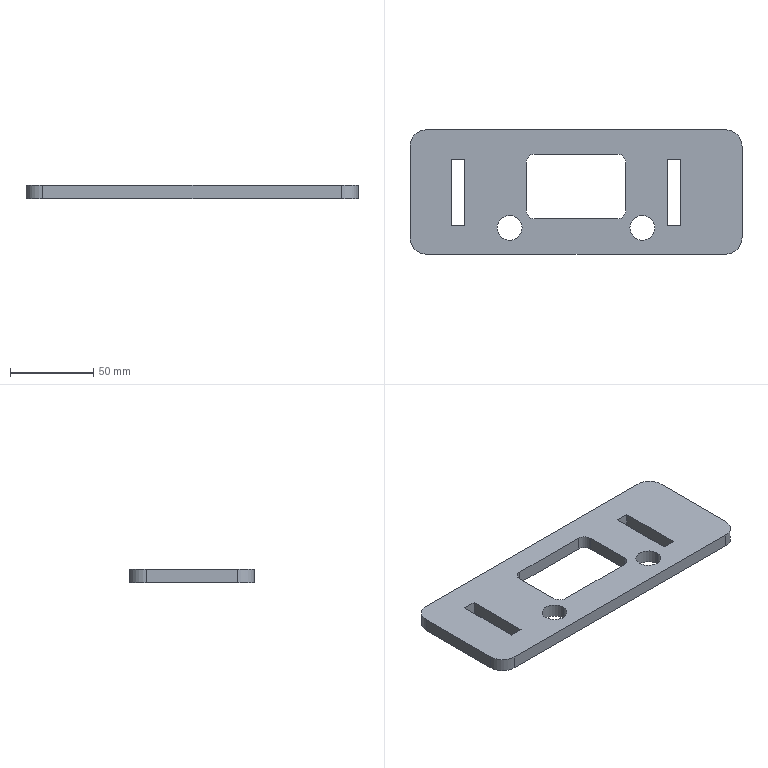Part | SolidWorks | features FlatPattern 1, SMBaseFlange 1, SheetMetal 1 | 1 solid | 30 faces | box 200 x 75 x 8 mm | volume 92818 mm3 | plane 18 | cylinder 12 | commonest cylinder face diameters 10 x4 15 x4 20 x4
STEP:
#1=CARTESIAN_POINT('',(32.5,147.915,8.));
#2=VERTEX_POINT('',#1);
#3=CARTESIAN_POINT('',(47.5,147.915,8.));
#4=VERTEX_POINT('',#3);
#5=CARTESIAN_POINT('',(40.,147.915,8.));
#6=DIRECTION('',(0.,0.,1.));
#7=DIRECTION('',(1.,0.,0.));
#8=AXIS2_PLACEMENT_3D('',#5,#6,#7);
#9=CIRCLE('',#8,7.5);
#10=EDGE_CURVE('',#2,#4,#9,.T.);
#11=ORIENTED_EDGE('',*,*,#10,.T.);
#12=CARTESIAN_POINT('',(47.5,147.915,0.));
#13=VERTEX_POINT('',#12);
#14=CARTESIAN_POINT('',(47.5,147.915,8.));
#15=DIRECTION('',(0.,0.,-1.));
#16=VECTOR('',#15,1000.);
#17=LINE('',#14,#16);
#18=EDGE_CURVE('',#4,#13,#17,.T.);
#19=ORIENTED_EDGE('',*,*,#18,.T.);
#20=CARTESIAN_POINT('',(32.5,147.915,0.));
#21=VERTEX_POINT('',#20);
#22=CARTESIAN_POINT('',(40.,147.915,0.));
#23=DIRECTION('',(0.,0.,1.));
#24=DIRECTION('',(1.,0.,0.));
#25=AXIS2_PLACEMENT_3D('',#22,#23,#24);
#26=CIRCLE('',#25,7.5);
#27=EDGE_CURVE('',#21,#13,#26,.T.);
#28=ORIENTED_EDGE('',*,*,#27,.F.);
#29=CARTESIAN_POINT('',(32.5,147.915,8.));
#30=DIRECTION('',(0.,0.,-1.));
#31=VECTOR('',#30,1000.);
#32=LINE('',#29,#31);
#33=EDGE_CURVE('',#2,#21,#32,.T.);
#34=ORIENTED_EDGE('',*,*,#33,.F.);
#35=EDGE_LOOP('',(#11,#19,#28,#34));
#36=FACE_OUTER_BOUND('',#35,.T.);
#37=CARTESIAN_POINT('',(40.,147.915,8.));
#38=DIRECTION('',(0.,0.,-1.));
#39=DIRECTION('',(-1.,0.,0.));
#40=AXIS2_PLACEMENT_3D('',#37,#38,#39);
#41=CYLINDRICAL_SURFACE('',#40,7.5);
#42=ADVANCED_FACE('',(#36),#41,.F.);
#43=CARTESIAN_POINT('',(-47.5,147.915,8.));
#44=VERTEX_POINT('',#43);
#45=CARTESIAN_POINT('',(-32.5,147.915,8.));
#46=VERTEX_POINT('',#45);
#47=CARTESIAN_POINT('',(-40.,147.915,8.));
#48=DIRECTION('',(0.,0.,1.));
#49=DIRECTION('',(1.,0.,0.));
#50=AXIS2_PLACEMENT_3D('',#47,#48,#49);
#51=CIRCLE('',#50,7.5);
#52=EDGE_CURVE('',#44,#46,#51,.T.);
#53=ORIENTED_EDGE('',*,*,#52,.T.);
#54=CARTESIAN_POINT('',(-32.5,147.915,0.));
#55=VERTEX_POINT('',#54);
#56=CARTESIAN_POINT('',(-32.5,147.915,8.));
#57=DIRECTION('',(0.,0.,-1.));
#58=VECTOR('',#57,1000.);
#59=LINE('',#56,#58);
#60=EDGE_CURVE('',#46,#55,#59,.T.);
#61=ORIENTED_EDGE('',*,*,#60,.T.);
#62=CARTESIAN_POINT('',(-47.5,147.915,0.));
#63=VERTEX_POINT('',#62);
#64=CARTESIAN_POINT('',(-40.,147.915,0.));
#65=DIRECTION('',(0.,0.,1.));
#66=DIRECTION('',(1.,0.,0.));
#67=AXIS2_PLACEMENT_3D('',#64,#65,#66);
#68=CIRCLE('',#67,7.5);
#69=EDGE_CURVE('',#63,#55,#68,.T.);
#70=ORIENTED_EDGE('',*,*,#69,.F.);
#71=CARTESIAN_POINT('',(-47.5,147.915,8.));
#72=DIRECTION('',(0.,0.,-1.));
#73=VECTOR('',#72,1000.);
#74=LINE('',#71,#73);
#75=EDGE_CURVE('',#44,#63,#74,.T.);
#76=ORIENTED_EDGE('',*,*,#75,.F.);
#77=EDGE_LOOP('',(#53,#61,#70,#76));
#78=FACE_OUTER_BOUND('',#77,.T.);
#79=CARTESIAN_POINT('',(-40.,147.915,8.));
#80=DIRECTION('',(0.,0.,-1.));
#81=DIRECTION('',(-1.,0.,0.));
#82=AXIS2_PLACEMENT_3D('',#79,#80,#81);
#83=CYLINDRICAL_SURFACE('',#82,7.5);
#84=ADVANCED_FACE('',(#78),#83,.F.);
#85=CARTESIAN_POINT('',(-75.,189.431,8.));
#86=VERTEX_POINT('',#85);
#87=CARTESIAN_POINT('',(-75.,149.431,8.));
#88=VERTEX_POINT('',#87);
#89=CARTESIAN_POINT('',(-75.,149.431,8.));
#90=DIRECTION('',(0.,-1.,0.));
#91=VECTOR('',#90,1000.);
#92=LINE('',#89,#91);
#93=EDGE_CURVE('',#86,#88,#92,.T.);
#94=ORIENTED_EDGE('',*,*,#93,.F.);
#95=CARTESIAN_POINT('',(-67.,189.431,8.));
#96=VERTEX_POINT('',#95);
#97=CARTESIAN_POINT('',(-75.,189.431,8.));
#98=DIRECTION('',(-1.,0.,0.));
#99=VECTOR('',#98,1000.);
#100=LINE('',#97,#99);
#101=EDGE_CURVE('',#96,#86,#100,.T.);
#102=ORIENTED_EDGE('',*,*,#101,.F.);
#103=CARTESIAN_POINT('',(-67.,149.431,8.));
#104=VERTEX_POINT('',#103);
#105=CARTESIAN_POINT('',(-67.,149.431,8.));
#106=DIRECTION('',(0.,1.,0.));
#107=VECTOR('',#106,1000.);
#108=LINE('',#105,#107);
#109=EDGE_CURVE('',#104,#96,#108,.T.);
#110=ORIENTED_EDGE('',*,*,#109,.F.);
#111=CARTESIAN_POINT('',(-75.,149.431,8.));
#112=DIRECTION('',(1.,0.,0.));
#113=VECTOR('',#112,1000.);
#114=LINE('',#111,#113);
#115=EDGE_CURVE('',#88,#104,#114,.T.);
#116=ORIENTED_EDGE('',*,*,#115,.F.);
#117=EDGE_LOOP('',(#94,#102,#110,#116));
#118=FACE_BOUND('',#117,.T.);
#119=ORIENTED_EDGE('',*,*,#10,.F.);
#120=CARTESIAN_POINT('',(40.,147.915,8.));
#121=DIRECTION('',(0.,0.,1.));
#122=DIRECTION('',(1.,0.,0.));
#123=AXIS2_PLACEMENT_3D('',#120,#121,#122);
#124=CIRCLE('',#123,7.5);
#125=EDGE_CURVE('',#4,#2,#124,.T.);
#126=ORIENTED_EDGE('',*,*,#125,.F.);
#127=EDGE_LOOP('',(#119,#126));
#128=FACE_BOUND('',#127,.T.);
#129=ORIENTED_EDGE('',*,*,#52,.F.);
#130=CARTESIAN_POINT('',(-40.,147.915,8.));
#131=DIRECTION('',(0.,0.,1.));
#132=DIRECTION('',(1.,0.,0.));
#133=AXIS2_PLACEMENT_3D('',#130,#131,#132);
#134=CIRCLE('',#133,7.5);
#135=EDGE_CURVE('',#46,#44,#134,.T.);
#136=ORIENTED_EDGE('',*,*,#135,.F.);
#137=EDGE_LOOP('',(#129,#136));
#138=FACE_BOUND('',#137,.T.);
#139=CARTESIAN_POINT('',(100.,197.08,8.));
#140=VERTEX_POINT('',#139);
#141=CARTESIAN_POINT('',(90.,207.08,8.));
#142=VERTEX_POINT('',#141);
#143=CARTESIAN_POINT('',(90.,197.08,8.));
#144=DIRECTION('',(0.,0.,1.));
#145=DIRECTION('',(-1.,0.,0.));
#146=AXIS2_PLACEMENT_3D('',#143,#144,#145);
#147=CIRCLE('',#146,10.);
#148=EDGE_CURVE('',#140,#142,#147,.T.);
#149=ORIENTED_EDGE('',*,*,#148,.T.);
#150=CARTESIAN_POINT('',(-90.,207.08,8.));
#151=VERTEX_POINT('',#150);
#152=CARTESIAN_POINT('',(-90.,207.08,8.));
#153=DIRECTION('',(-1.,0.,0.));
#154=VECTOR('',#153,1000.);
#155=LINE('',#152,#154);
#156=EDGE_CURVE('',#142,#151,#155,.T.);
#157=ORIENTED_EDGE('',*,*,#156,.T.);
#158=CARTESIAN_POINT('',(-100.,197.08,8.));
#159=VERTEX_POINT('',#158);
#160=CARTESIAN_POINT('',(-90.,197.08,8.));
#161=DIRECTION('',(0.,0.,1.));
#162=DIRECTION('',(-1.,0.,0.));
#163=AXIS2_PLACEMENT_3D('',#160,#161,#162);
#164=CIRCLE('',#163,10.);
#165=EDGE_CURVE('',#151,#159,#164,.T.);
#166=ORIENTED_EDGE('',*,*,#165,.T.);
#167=CARTESIAN_POINT('',(-100.,142.08,8.));
#168=VERTEX_POINT('',#167);
#169=CARTESIAN_POINT('',(-100.,142.08,8.));
#170=DIRECTION('',(0.,-1.,0.));
#171=VECTOR('',#170,1000.);
#172=LINE('',#169,#171);
#173=EDGE_CURVE('',#159,#168,#172,.T.);
#174=ORIENTED_EDGE('',*,*,#173,.T.);
#175=CARTESIAN_POINT('',(-90.,132.08,8.));
#176=VERTEX_POINT('',#175);
#177=CARTESIAN_POINT('',(-90.,142.08,8.));
#178=DIRECTION('',(0.,0.,1.));
#179=DIRECTION('',(-1.,0.,0.));
#180=AXIS2_PLACEMENT_3D('',#177,#178,#179);
#181=CIRCLE('',#180,10.);
#182=EDGE_CURVE('',#168,#176,#181,.T.);
#183=ORIENTED_EDGE('',*,*,#182,.T.);
#184=CARTESIAN_POINT('',(90.,132.08,8.));
#185=VERTEX_POINT('',#184);
#186=CARTESIAN_POINT('',(90.,132.08,8.));
#187=DIRECTION('',(1.,0.,0.));
#188=VECTOR('',#187,1000.);
#189=LINE('',#186,#188);
#190=EDGE_CURVE('',#176,#185,#189,.T.);
#191=ORIENTED_EDGE('',*,*,#190,.T.);
#192=CARTESIAN_POINT('',(100.,142.08,8.));
#193=VERTEX_POINT('',#192);
#194=CARTESIAN_POINT('',(90.,142.08,8.));
#195=DIRECTION('',(0.,0.,1.));
#196=DIRECTION('',(1.,0.,0.));
#197=AXIS2_PLACEMENT_3D('',#194,#195,#196);
#198=CIRCLE('',#197,10.);
#199=EDGE_CURVE('',#185,#193,#198,.T.);
#200=ORIENTED_EDGE('',*,*,#199,.T.);
#201=CARTESIAN_POINT('',(100.,197.08,8.));
#202=DIRECTION('',(0.,1.,0.));
#203=VECTOR('',#202,1000.);
#204=LINE('',#201,#203);
#205=EDGE_CURVE('',#193,#140,#204,.T.);
#206=ORIENTED_EDGE('',*,*,#205,.T.);
#207=EDGE_LOOP('',(#149,#157,#166,#174,#183,#191,#200,#206));
#208=FACE_OUTER_BOUND('',#207,.T.);
#209=CARTESIAN_POINT('',(-25.,192.415,8.));
#210=VERTEX_POINT('',#209);
#211=CARTESIAN_POINT('',(-30.,187.415,8.));
#212=VERTEX_POINT('',#211);
#213=CARTESIAN_POINT('',(-25.,187.415,8.));
#214=DIRECTION('',(0.,0.,1.));
#215=DIRECTION('',(-1.,0.,0.));
#216=AXIS2_PLACEMENT_3D('',#213,#214,#215);
#217=CIRCLE('',#216,5.);
#218=EDGE_CURVE('',#210,#212,#217,.T.);
#219=ORIENTED_EDGE('',*,*,#218,.F.);
#220=CARTESIAN_POINT('',(25.,192.415,8.));
#221=VERTEX_POINT('',#220);
#222=CARTESIAN_POINT('',(-25.,192.415,8.));
#223=DIRECTION('',(-1.,0.,0.));
#224=VECTOR('',#223,1000.);
#225=LINE('',#222,#224);
#226=EDGE_CURVE('',#221,#210,#225,.T.);
#227=ORIENTED_EDGE('',*,*,#226,.F.);
#228=CARTESIAN_POINT('',(30.,187.415,8.));
#229=VERTEX_POINT('',#228);
#230=CARTESIAN_POINT('',(25.,187.415,8.));
#231=DIRECTION('',(0.,0.,1.));
#232=DIRECTION('',(1.,0.,0.));
#233=AXIS2_PLACEMENT_3D('',#230,#231,#232);
#234=CIRCLE('',#233,5.);
#235=EDGE_CURVE('',#229,#221,#234,.T.);
#236=ORIENTED_EDGE('',*,*,#235,.F.);
#237=CARTESIAN_POINT('',(30.,158.415,8.));
#238=VERTEX_POINT('',#237);
#239=CARTESIAN_POINT('',(30.,158.415,8.));
#240=DIRECTION('',(0.,1.,0.));
#241=VECTOR('',#240,1000.);
#242=LINE('',#239,#241);
#243=EDGE_CURVE('',#238,#229,#242,.T.);
#244=ORIENTED_EDGE('',*,*,#243,.F.);
#245=CARTESIAN_POINT('',(25.,153.415,8.));
#246=VERTEX_POINT('',#245);
#247=CARTESIAN_POINT('',(25.,158.415,8.));
#248=DIRECTION('',(0.,0.,1.));
#249=DIRECTION('',(1.,0.,0.));
#250=AXIS2_PLACEMENT_3D('',#247,#248,#249);
#251=CIRCLE('',#250,5.);
#252=EDGE_CURVE('',#246,#238,#251,.T.);
#253=ORIENTED_EDGE('',*,*,#252,.F.);
#254=CARTESIAN_POINT('',(-25.,153.415,8.));
#255=VERTEX_POINT('',#254);
#256=CARTESIAN_POINT('',(-25.,153.415,8.));
#257=DIRECTION('',(1.,0.,0.));
#258=VECTOR('',#257,1000.);
#259=LINE('',#256,#258);
#260=EDGE_CURVE('',#255,#246,#259,.T.);
#261=ORIENTED_EDGE('',*,*,#260,.F.);
#262=CARTESIAN_POINT('',(-30.,158.415,8.));
#263=VERTEX_POINT('',#262);
#264=CARTESIAN_POINT('',(-25.,158.415,8.));
#265=DIRECTION('',(0.,0.,1.));
#266=DIRECTION('',(1.,0.,0.));
#267=AXIS2_PLACEMENT_3D('',#264,#265,#266);
#268=CIRCLE('',#267,5.);
#269=EDGE_CURVE('',#263,#255,#268,.T.);
#270=ORIENTED_EDGE('',*,*,#269,.F.);
#271=CARTESIAN_POINT('',(-30.,187.415,8.));
#272=DIRECTION('',(0.,-1.,0.));
#273=VECTOR('',#272,1000.);
#274=LINE('',#271,#273);
#275=EDGE_CURVE('',#212,#263,#274,.T.);
#276=ORIENTED_EDGE('',*,*,#275,.F.);
#277=EDGE_LOOP('',(#219,#227,#236,#244,#253,#261,#270,#276));
#278=FACE_BOUND('',#277,.T.);
#279=CARTESIAN_POINT('',(55.,189.431,8.));
#280=VERTEX_POINT('',#279);
#281=CARTESIAN_POINT('',(55.,149.431,8.));
#282=VERTEX_POINT('',#281);
#283=CARTESIAN_POINT('',(55.,149.431,8.));
#284=DIRECTION('',(0.,-1.,0.));
#285=VECTOR('',#284,1000.);
#286=LINE('',#283,#285);
#287=EDGE_CURVE('',#280,#282,#286,.T.);
#288=ORIENTED_EDGE('',*,*,#287,.F.);
#289=CARTESIAN_POINT('',(63.,189.431,8.));
#290=VERTEX_POINT('',#289);
#291=CARTESIAN_POINT('',(55.,189.431,8.));
#292=DIRECTION('',(-1.,0.,0.));
#293=VECTOR('',#292,1000.);
#294=LINE('',#291,#293);
#295=EDGE_CURVE('',#290,#280,#294,.T.);
#296=ORIENTED_EDGE('',*,*,#295,.F.);
#297=CARTESIAN_POINT('',(63.,149.431,8.));
#298=VERTEX_POINT('',#297);
#299=CARTESIAN_POINT('',(63.,149.431,8.));
#300=DIRECTION('',(0.,1.,0.));
#301=VECTOR('',#300,1000.);
#302=LINE('',#299,#301);
#303=EDGE_CURVE('',#298,#290,#302,.T.);
#304=ORIENTED_EDGE('',*,*,#303,.F.);
#305=CARTESIAN_POINT('',(55.,149.431,8.));
#306=DIRECTION('',(1.,0.,0.));
#307=VECTOR('',#306,1000.);
#308=LINE('',#305,#307);
#309=EDGE_CURVE('',#282,#298,#308,.T.);
#310=ORIENTED_EDGE('',*,*,#309,.F.);
#311=EDGE_LOOP('',(#288,#296,#304,#310));
#312=FACE_BOUND('',#311,.T.);
#313=CARTESIAN_POINT('',(90.,197.08,8.));
#314=DIRECTION('',(0.,0.,-1.));
#315=DIRECTION('',(-1.,0.,0.));
#316=AXIS2_PLACEMENT_3D('',#313,#314,#315);
#317=PLANE('',#316);
#318=ADVANCED_FACE('',(#118,#128,#138,#208,#278,#312),#317,.F.);
#319=ORIENTED_EDGE('',*,*,#69,.T.);
#320=CARTESIAN_POINT('',(-40.,147.915,0.));
#321=DIRECTION('',(0.,0.,1.));
#322=DIRECTION('',(1.,0.,0.));
#323=AXIS2_PLACEMENT_3D('',#320,#321,#322);
#324=CIRCLE('',#323,7.5);
#325=EDGE_CURVE('',#55,#63,#324,.T.);
#326=ORIENTED_EDGE('',*,*,#325,.T.);
#327=EDGE_LOOP('',(#319,#326));
#328=FACE_BOUND('',#327,.T.);
#329=CARTESIAN_POINT('',(100.,197.08,0.));
#330=VERTEX_POINT('',#329);
#331=CARTESIAN_POINT('',(90.,207.08,0.));
#332=VERTEX_POINT('',#331);
#333=CARTESIAN_POINT('',(90.,197.08,0.));
#334=DIRECTION('',(0.,0.,1.));
#335=DIRECTION('',(-1.,0.,0.));
#336=AXIS2_PLACEMENT_3D('',#333,#334,#335);
#337=CIRCLE('',#336,10.);
#338=EDGE_CURVE('',#330,#332,#337,.T.);
#339=ORIENTED_EDGE('',*,*,#338,.F.);
#340=CARTESIAN_POINT('',(100.,142.08,0.));
#341=VERTEX_POINT('',#340);
#342=CARTESIAN_POINT('',(100.,197.08,0.));
#343=DIRECTION('',(0.,1.,0.));
#344=VECTOR('',#343,1000.);
#345=LINE('',#342,#344);
#346=EDGE_CURVE('',#341,#330,#345,.T.);
#347=ORIENTED_EDGE('',*,*,#346,.F.);
#348=CARTESIAN_POINT('',(90.,132.08,0.));
#349=VERTEX_POINT('',#348);
#350=CARTESIAN_POINT('',(90.,142.08,0.));
#351=DIRECTION('',(0.,0.,1.));
#352=DIRECTION('',(1.,0.,0.));
#353=AXIS2_PLACEMENT_3D('',#350,#351,#352);
#354=CIRCLE('',#353,10.);
#355=EDGE_CURVE('',#349,#341,#354,.T.);
#356=ORIENTED_EDGE('',*,*,#355,.F.);
#357=CARTESIAN_POINT('',(-90.,132.08,0.));
#358=VERTEX_POINT('',#357);
#359=CARTESIAN_POINT('',(90.,132.08,0.));
#360=DIRECTION('',(1.,0.,0.));
#361=VECTOR('',#360,1000.);
#362=LINE('',#359,#361);
#363=EDGE_CURVE('',#358,#349,#362,.T.);
#364=ORIENTED_EDGE('',*,*,#363,.F.);
#365=CARTESIAN_POINT('',(-100.,142.08,0.));
#366=VERTEX_POINT('',#365);
#367=CARTESIAN_POINT('',(-90.,142.08,0.));
#368=DIRECTION('',(0.,0.,1.));
#369=DIRECTION('',(-1.,0.,0.));
#370=AXIS2_PLACEMENT_3D('',#367,#368,#369);
#371=CIRCLE('',#370,10.);
#372=EDGE_CURVE('',#366,#358,#371,.T.);
#373=ORIENTED_EDGE('',*,*,#372,.F.);
#374=CARTESIAN_POINT('',(-100.,197.08,0.));
#375=VERTEX_POINT('',#374);
#376=CARTESIAN_POINT('',(-100.,142.08,0.));
#377=DIRECTION('',(0.,-1.,0.));
#378=VECTOR('',#377,1000.);
#379=LINE('',#376,#378);
#380=EDGE_CURVE('',#375,#366,#379,.T.);
#381=ORIENTED_EDGE('',*,*,#380,.F.);
#382=CARTESIAN_POINT('',(-90.,207.08,0.));
#383=VERTEX_POINT('',#382);
#384=CARTESIAN_POINT('',(-90.,197.08,0.));
#385=DIRECTION('',(0.,0.,1.));
#386=DIRECTION('',(-1.,0.,0.));
#387=AXIS2_PLACEMENT_3D('',#384,#385,#386);
#388=CIRCLE('',#387,10.);
#389=EDGE_CURVE('',#383,#375,#388,.T.);
#390=ORIENTED_EDGE('',*,*,#389,.F.);
#391=CARTESIAN_POINT('',(-90.,207.08,0.));
#392=DIRECTION('',(-1.,0.,0.));
#393=VECTOR('',#392,1000.);
#394=LINE('',#391,#393);
#395=EDGE_CURVE('',#332,#383,#394,.T.);
#396=ORIENTED_EDGE('',*,*,#395,.F.);
#397=EDGE_LOOP('',(#339,#347,#356,#364,#373,#381,#390,#396));
#398=FACE_OUTER_BOUND('',#397,.T.);
#399=ORIENTED_EDGE('',*,*,#27,.T.);
#400=CARTESIAN_POINT('',(40.,147.915,0.));
#401=DIRECTION('',(0.,0.,1.));
#402=DIRECTION('',(1.,0.,0.));
#403=AXIS2_PLACEMENT_3D('',#400,#401,#402);
#404=CIRCLE('',#403,7.5);
#405=EDGE_CURVE('',#13,#21,#404,.T.);
#406=ORIENTED_EDGE('',*,*,#405,.T.);
#407=EDGE_LOOP('',(#399,#406));
#408=FACE_BOUND('',#407,.T.);
#409=CARTESIAN_POINT('',(25.,192.415,0.));
#410=VERTEX_POINT('',#409);
#411=CARTESIAN_POINT('',(-25.,192.415,0.));
#412=VERTEX_POINT('',#411);
#413=CARTESIAN_POINT('',(-25.,192.415,0.));
#414=DIRECTION('',(-1.,0.,0.));
#415=VECTOR('',#414,1000.);
#416=LINE('',#413,#415);
#417=EDGE_CURVE('',#410,#412,#416,.T.);
#418=ORIENTED_EDGE('',*,*,#417,.T.);
#419=CARTESIAN_POINT('',(-30.,187.415,0.));
#420=VERTEX_POINT('',#419);
#421=CARTESIAN_POINT('',(-25.,187.415,0.));
#422=DIRECTION('',(0.,0.,1.));
#423=DIRECTION('',(-1.,0.,0.));
#424=AXIS2_PLACEMENT_3D('',#421,#422,#423);
#425=CIRCLE('',#424,5.);
#426=EDGE_CURVE('',#412,#420,#425,.T.);
#427=ORIENTED_EDGE('',*,*,#426,.T.);
#428=CARTESIAN_POINT('',(-30.,158.415,0.));
#429=VERTEX_POINT('',#428);
#430=CARTESIAN_POINT('',(-30.,187.415,0.));
#431=DIRECTION('',(0.,-1.,0.));
#432=VECTOR('',#431,1000.);
#433=LINE('',#430,#432);
#434=EDGE_CURVE('',#420,#429,#433,.T.);
#435=ORIENTED_EDGE('',*,*,#434,.T.);
#436=CARTESIAN_POINT('',(-25.,153.415,0.));
#437=VERTEX_POINT('',#436);
#438=CARTESIAN_POINT('',(-25.,158.415,0.));
#439=DIRECTION('',(0.,0.,1.));
#440=DIRECTION('',(1.,0.,0.));
#441=AXIS2_PLACEMENT_3D('',#438,#439,#440);
#442=CIRCLE('',#441,5.);
#443=EDGE_CURVE('',#429,#437,#442,.T.);
#444=ORIENTED_EDGE('',*,*,#443,.T.);
#445=CARTESIAN_POINT('',(25.,153.415,0.));
#446=VERTEX_POINT('',#445);
#447=CARTESIAN_POINT('',(-25.,153.415,0.));
#448=DIRECTION('',(1.,0.,0.));
#449=VECTOR('',#448,1000.);
#450=LINE('',#447,#449);
#451=EDGE_CURVE('',#437,#446,#450,.T.);
#452=ORIENTED_EDGE('',*,*,#451,.T.);
#453=CARTESIAN_POINT('',(30.,158.415,0.));
#454=VERTEX_POINT('',#453);
#455=CARTESIAN_POINT('',(25.,158.415,0.));
#456=DIRECTION('',(0.,0.,1.));
#457=DIRECTION('',(1.,0.,0.));
#458=AXIS2_PLACEMENT_3D('',#455,#456,#457);
#459=CIRCLE('',#458,5.);
#460=EDGE_CURVE('',#446,#454,#459,.T.);
#461=ORIENTED_EDGE('',*,*,#460,.T.);
#462=CARTESIAN_POINT('',(30.,187.415,0.));
#463=VERTEX_POINT('',#462);
#464=CARTESIAN_POINT('',(30.,158.415,0.));
#465=DIRECTION('',(0.,1.,0.));
#466=VECTOR('',#465,1000.);
#467=LINE('',#464,#466);
#468=EDGE_CURVE('',#454,#463,#467,.T.);
#469=ORIENTED_EDGE('',*,*,#468,.T.);
#470=CARTESIAN_POINT('',(25.,187.415,0.));
#471=DIRECTION('',(0.,0.,1.));
#472=DIRECTION('',(1.,0.,0.));
#473=AXIS2_PLACEMENT_3D('',#470,#471,#472);
#474=CIRCLE('',#473,5.);
#475=EDGE_CURVE('',#463,#410,#474,.T.);
#476=ORIENTED_EDGE('',*,*,#475,.T.);
#477=EDGE_LOOP('',(#418,#427,#435,#444,#452,#461,#469,#476));
#478=FACE_BOUND('',#477,.T.);
#479=CARTESIAN_POINT('',(-67.,189.431,0.));
#480=VERTEX_POINT('',#479);
#481=CARTESIAN_POINT('',(-75.,189.431,0.));
#482=VERTEX_POINT('',#481);
#483=CARTESIAN_POINT('',(-75.,189.431,0.));
#484=DIRECTION('',(-1.,0.,0.));
#485=VECTOR('',#484,1000.);
#486=LINE('',#483,#485);
#487=EDGE_CURVE('',#480,#482,#486,.T.);
#488=ORIENTED_EDGE('',*,*,#487,.T.);
#489=CARTESIAN_POINT('',(-75.,149.431,0.));
#490=VERTEX_POINT('',#489);
#491=CARTESIAN_POINT('',(-75.,149.431,0.));
#492=DIRECTION('',(0.,-1.,0.));
#493=VECTOR('',#492,1000.);
#494=LINE('',#491,#493);
#495=EDGE_CURVE('',#482,#490,#494,.T.);
#496=ORIENTED_EDGE('',*,*,#495,.T.);
#497=CARTESIAN_POINT('',(-67.,149.431,0.));
#498=VERTEX_POINT('',#497);
#499=CARTESIAN_POINT('',(-75.,149.431,0.));
#500=DIRECTION('',(1.,0.,0.));
#501=VECTOR('',#500,1000.);
#502=LINE('',#499,#501);
#503=EDGE_CURVE('',#490,#498,#502,.T.);
#504=ORIENTED_EDGE('',*,*,#503,.T.);
#505=CARTESIAN_POINT('',(-67.,149.431,0.));
#506=DIRECTION('',(0.,1.,0.));
#507=VECTOR('',#506,1000.);
#508=LINE('',#505,#507);
#509=EDGE_CURVE('',#498,#480,#508,.T.);
#510=ORIENTED_EDGE('',*,*,#509,.T.);
#511=EDGE_LOOP('',(#488,#496,#504,#510));
#512=FACE_BOUND('',#511,.T.);
#513=CARTESIAN_POINT('',(63.,189.431,0.));
#514=VERTEX_POINT('',#513);
#515=CARTESIAN_POINT('',(55.,189.431,0.));
#516=VERTEX_POINT('',#515);
#517=CARTESIAN_POINT('',(55.,189.431,0.));
#518=DIRECTION('',(-1.,0.,0.));
#519=VECTOR('',#518,1000.);
#520=LINE('',#517,#519);
#521=EDGE_CURVE('',#514,#516,#520,.T.);
#522=ORIENTED_EDGE('',*,*,#521,.T.);
#523=CARTESIAN_POINT('',(55.,149.431,0.));
#524=VERTEX_POINT('',#523);
#525=CARTESIAN_POINT('',(55.,149.431,0.));
#526=DIRECTION('',(0.,-1.,0.));
#527=VECTOR('',#526,1000.);
#528=LINE('',#525,#527);
#529=EDGE_CURVE('',#516,#524,#528,.T.);
#530=ORIENTED_EDGE('',*,*,#529,.T.);
#531=CARTESIAN_POINT('',(63.,149.431,0.));
#532=VERTEX_POINT('',#531);
#533=CARTESIAN_POINT('',(55.,149.431,0.));
#534=DIRECTION('',(1.,0.,0.));
#535=VECTOR('',#534,1000.);
#536=LINE('',#533,#535);
#537=EDGE_CURVE('',#524,#532,#536,.T.);
#538=ORIENTED_EDGE('',*,*,#537,.T.);
#539=CARTESIAN_POINT('',(63.,149.431,0.));
#540=DIRECTION('',(0.,1.,0.));
#541=VECTOR('',#540,1000.);
#542=LINE('',#539,#541);
#543=EDGE_CURVE('',#532,#514,#542,.T.);
#544=ORIENTED_EDGE('',*,*,#543,.T.);
#545=EDGE_LOOP('',(#522,#530,#538,#544));
#546=FACE_BOUND('',#545,.T.);
#547=CARTESIAN_POINT('',(90.,197.08,0.));
#548=DIRECTION('',(0.,0.,-1.));
#549=DIRECTION('',(-1.,0.,0.));
#550=AXIS2_PLACEMENT_3D('',#547,#548,#549);
#551=PLANE('',#550);
#552=ADVANCED_FACE('',(#328,#398,#408,#478,#512,#546),#551,.T.);
#553=ORIENTED_EDGE('',*,*,#338,.T.);
#554=CARTESIAN_POINT('',(90.,207.08,8.));
#555=DIRECTION('',(0.,0.,-1.));
#556=VECTOR('',#555,1000.);
#557=LINE('',#554,#556);
#558=EDGE_CURVE('',#142,#332,#557,.T.);
#559=ORIENTED_EDGE('',*,*,#558,.F.);
#560=ORIENTED_EDGE('',*,*,#148,.F.);
#561=CARTESIAN_POINT('',(100.,197.08,8.));
#562=DIRECTION('',(0.,0.,-1.));
#563=VECTOR('',#562,1000.);
#564=LINE('',#561,#563);
#565=EDGE_CURVE('',#140,#330,#564,.T.);
#566=ORIENTED_EDGE('',*,*,#565,.T.);
#567=EDGE_LOOP('',(#553,#559,#560,#566));
#568=FACE_OUTER_BOUND('',#567,.T.);
#569=CARTESIAN_POINT('',(90.,197.08,8.));
#570=DIRECTION('',(0.,0.,-1.));
#571=DIRECTION('',(-1.,0.,0.));
#572=AXIS2_PLACEMENT_3D('',#569,#570,#571);
#573=CYLINDRICAL_SURFACE('',#572,10.);
#574=ADVANCED_FACE('',(#568),#573,.T.);
#575=ORIENTED_EDGE('',*,*,#395,.T.);
#576=CARTESIAN_POINT('',(-90.,207.08,8.));
#577=DIRECTION('',(0.,0.,-1.));
#578=VECTOR('',#577,1000.);
#579=LINE('',#576,#578);
#580=EDGE_CURVE('',#151,#383,#579,.T.);
#581=ORIENTED_EDGE('',*,*,#580,.F.);
#582=ORIENTED_EDGE('',*,*,#156,.F.);
#583=ORIENTED_EDGE('',*,*,#558,.T.);
#584=EDGE_LOOP('',(#575,#581,#582,#583));
#585=FACE_OUTER_BOUND('',#584,.T.);
#586=CARTESIAN_POINT('',(-90.,207.08,8.));
#587=DIRECTION('',(0.,-1.,0.));
#588=DIRECTION('',(0.,0.,-1.));
#589=AXIS2_PLACEMENT_3D('',#586,#587,#588);
#590=PLANE('',#589);
#591=ADVANCED_FACE('',(#585),#590,.F.);
#592=ORIENTED_EDGE('',*,*,#389,.T.);
#593=CARTESIAN_POINT('',(-100.,197.08,8.));
#594=DIRECTION('',(0.,0.,-1.));
#595=VECTOR('',#594,1000.);
#596=LINE('',#593,#595);
#597=EDGE_CURVE('',#159,#375,#596,.T.);
#598=ORIENTED_EDGE('',*,*,#597,.F.);
#599=ORIENTED_EDGE('',*,*,#165,.F.);
#600=ORIENTED_EDGE('',*,*,#580,.T.);
#601=EDGE_LOOP('',(#592,#598,#599,#600));
#602=FACE_OUTER_BOUND('',#601,.T.);
#603=CARTESIAN_POINT('',(-90.,197.08,8.));
#604=DIRECTION('',(0.,0.,-1.));
#605=DIRECTION('',(-1.,0.,0.));
#606=AXIS2_PLACEMENT_3D('',#603,#604,#605);
#607=CYLINDRICAL_SURFACE('',#606,10.);
#608=ADVANCED_FACE('',(#602),#607,.T.);
#609=ORIENTED_EDGE('',*,*,#380,.T.);
#610=CARTESIAN_POINT('',(-100.,142.08,8.));
#611=DIRECTION('',(0.,0.,-1.));
#612=VECTOR('',#611,1000.);
#613=LINE('',#610,#612);
#614=EDGE_CURVE('',#168,#366,#613,.T.);
#615=ORIENTED_EDGE('',*,*,#614,.F.);
#616=ORIENTED_EDGE('',*,*,#173,.F.);
#617=ORIENTED_EDGE('',*,*,#597,.T.);
#618=EDGE_LOOP('',(#609,#615,#616,#617));
#619=FACE_OUTER_BOUND('',#618,.T.);
#620=CARTESIAN_POINT('',(-100.,142.08,8.));
#621=DIRECTION('',(1.,0.,0.));
#622=DIRECTION('',(0.,1.,0.));
#623=AXIS2_PLACEMENT_3D('',#620,#621,#622);
#624=PLANE('',#623);
#625=ADVANCED_FACE('',(#619),#624,.F.);
#626=ORIENTED_EDGE('',*,*,#372,.T.);
#627=CARTESIAN_POINT('',(-90.,132.08,8.));
#628=DIRECTION('',(0.,0.,-1.));
#629=VECTOR('',#628,1000.);
#630=LINE('',#627,#629);
#631=EDGE_CURVE('',#176,#358,#630,.T.);
#632=ORIENTED_EDGE('',*,*,#631,.F.);
#633=ORIENTED_EDGE('',*,*,#182,.F.);
#634=ORIENTED_EDGE('',*,*,#614,.T.);
#635=EDGE_LOOP('',(#626,#632,#633,#634));
#636=FACE_OUTER_BOUND('',#635,.T.);
#637=CARTESIAN_POINT('',(-90.,142.08,8.));
#638=DIRECTION('',(0.,0.,-1.));
#639=DIRECTION('',(-1.,0.,0.));
#640=AXIS2_PLACEMENT_3D('',#637,#638,#639);
#641=CYLINDRICAL_SURFACE('',#640,10.);
#642=ADVANCED_FACE('',(#636),#641,.T.);
#643=ORIENTED_EDGE('',*,*,#363,.T.);
#644=CARTESIAN_POINT('',(90.,132.08,8.));
#645=DIRECTION('',(0.,0.,-1.));
#646=VECTOR('',#645,1000.);
#647=LINE('',#644,#646);
#648=EDGE_CURVE('',#185,#349,#647,.T.);
#649=ORIENTED_EDGE('',*,*,#648,.F.);
#650=ORIENTED_EDGE('',*,*,#190,.F.);
#651=ORIENTED_EDGE('',*,*,#631,.T.);
#652=EDGE_LOOP('',(#643,#649,#650,#651));
#653=FACE_OUTER_BOUND('',#652,.T.);
#654=CARTESIAN_POINT('',(90.,132.08,8.));
#655=DIRECTION('',(0.,1.,0.));
#656=DIRECTION('',(0.,0.,1.));
#657=AXIS2_PLACEMENT_3D('',#654,#655,#656);
#658=PLANE('',#657);
#659=ADVANCED_FACE('',(#653),#658,.F.);
#660=ORIENTED_EDGE('',*,*,#355,.T.);
#661=CARTESIAN_POINT('',(100.,142.08,8.));
#662=DIRECTION('',(0.,0.,-1.));
#663=VECTOR('',#662,1000.);
#664=LINE('',#661,#663);
#665=EDGE_CURVE('',#193,#341,#664,.T.);
#666=ORIENTED_EDGE('',*,*,#665,.F.);
#667=ORIENTED_EDGE('',*,*,#199,.F.);
#668=ORIENTED_EDGE('',*,*,#648,.T.);
#669=EDGE_LOOP('',(#660,#666,#667,#668));
#670=FACE_OUTER_BOUND('',#669,.T.);
#671=CARTESIAN_POINT('',(90.,142.08,8.));
#672=DIRECTION('',(0.,0.,-1.));
#673=DIRECTION('',(-1.,0.,0.));
#674=AXIS2_PLACEMENT_3D('',#671,#672,#673);
#675=CYLINDRICAL_SURFACE('',#674,10.);
#676=ADVANCED_FACE('',(#670),#675,.T.);
#677=ORIENTED_EDGE('',*,*,#346,.T.);
#678=ORIENTED_EDGE('',*,*,#565,.F.);
#679=ORIENTED_EDGE('',*,*,#205,.F.);
#680=ORIENTED_EDGE('',*,*,#665,.T.);
#681=EDGE_LOOP('',(#677,#678,#679,#680));
#682=FACE_OUTER_BOUND('',#681,.T.);
#683=CARTESIAN_POINT('',(100.,197.08,8.));
#684=DIRECTION('',(-1.,0.,0.));
#685=DIRECTION('',(0.,-1.,0.));
#686=AXIS2_PLACEMENT_3D('',#683,#684,#685);
#687=PLANE('',#686);
#688=ADVANCED_FACE('',(#682),#687,.F.);
#689=ORIENTED_EDGE('',*,*,#60,.F.);
#690=ORIENTED_EDGE('',*,*,#135,.T.);
#691=ORIENTED_EDGE('',*,*,#75,.T.);
#692=ORIENTED_EDGE('',*,*,#325,.F.);
#693=EDGE_LOOP('',(#689,#690,#691,#692));
#694=FACE_OUTER_BOUND('',#693,.T.);
#695=CARTESIAN_POINT('',(-40.,147.915,8.));
#696=DIRECTION('',(0.,0.,-1.));
#697=DIRECTION('',(-1.,0.,0.));
#698=AXIS2_PLACEMENT_3D('',#695,#696,#697);
#699=CYLINDRICAL_SURFACE('',#698,7.5);
#700=ADVANCED_FACE('',(#694),#699,.F.);
#701=ORIENTED_EDGE('',*,*,#18,.F.);
#702=ORIENTED_EDGE('',*,*,#125,.T.);
#703=ORIENTED_EDGE('',*,*,#33,.T.);
#704=ORIENTED_EDGE('',*,*,#405,.F.);
#705=EDGE_LOOP('',(#701,#702,#703,#704));
#706=FACE_OUTER_BOUND('',#705,.T.);
#707=CARTESIAN_POINT('',(40.,147.915,8.));
#708=DIRECTION('',(0.,0.,-1.));
#709=DIRECTION('',(-1.,0.,0.));
#710=AXIS2_PLACEMENT_3D('',#707,#708,#709);
#711=CYLINDRICAL_SURFACE('',#710,7.5);
#712=ADVANCED_FACE('',(#706),#711,.F.);
#713=ORIENTED_EDGE('',*,*,#426,.F.);
#714=CARTESIAN_POINT('',(-25.,192.415,8.));
#715=DIRECTION('',(0.,0.,-1.));
#716=VECTOR('',#715,1000.);
#717=LINE('',#714,#716);
#718=EDGE_CURVE('',#210,#412,#717,.T.);
#719=ORIENTED_EDGE('',*,*,#718,.F.);
#720=ORIENTED_EDGE('',*,*,#218,.T.);
#721=CARTESIAN_POINT('',(-30.,187.415,8.));
#722=DIRECTION('',(0.,0.,-1.));
#723=VECTOR('',#722,1000.);
#724=LINE('',#721,#723);
#725=EDGE_CURVE('',#212,#420,#724,.T.);
#726=ORIENTED_EDGE('',*,*,#725,.T.);
#727=EDGE_LOOP('',(#713,#719,#720,#726));
#728=FACE_OUTER_BOUND('',#727,.T.);
#729=CARTESIAN_POINT('',(-25.,187.415,8.));
#730=DIRECTION('',(0.,0.,-1.));
#731=DIRECTION('',(-1.,0.,0.));
#732=AXIS2_PLACEMENT_3D('',#729,#730,#731);
#733=CYLINDRICAL_SURFACE('',#732,5.);
#734=ADVANCED_FACE('',(#728),#733,.F.);
#735=ORIENTED_EDGE('',*,*,#434,.F.);
#736=ORIENTED_EDGE('',*,*,#725,.F.);
#737=ORIENTED_EDGE('',*,*,#275,.T.);
#738=CARTESIAN_POINT('',(-30.,158.415,8.));
#739=DIRECTION('',(0.,0.,-1.));
#740=VECTOR('',#739,1000.);
#741=LINE('',#738,#740);
#742=EDGE_CURVE('',#263,#429,#741,.T.);
#743=ORIENTED_EDGE('',*,*,#742,.T.);
#744=EDGE_LOOP('',(#735,#736,#737,#743));
#745=FACE_OUTER_BOUND('',#744,.T.);
#746=CARTESIAN_POINT('',(-30.,187.415,8.));
#747=DIRECTION('',(1.,0.,0.));
#748=DIRECTION('',(0.,1.,0.));
#749=AXIS2_PLACEMENT_3D('',#746,#747,#748);
#750=PLANE('',#749);
#751=ADVANCED_FACE('',(#745),#750,.T.);
#752=ORIENTED_EDGE('',*,*,#443,.F.);
#753=ORIENTED_EDGE('',*,*,#742,.F.);
#754=ORIENTED_EDGE('',*,*,#269,.T.);
#755=CARTESIAN_POINT('',(-25.,153.415,8.));
#756=DIRECTION('',(0.,0.,-1.));
#757=VECTOR('',#756,1000.);
#758=LINE('',#755,#757);
#759=EDGE_CURVE('',#255,#437,#758,.T.);
#760=ORIENTED_EDGE('',*,*,#759,.T.);
#761=EDGE_LOOP('',(#752,#753,#754,#760));
#762=FACE_OUTER_BOUND('',#761,.T.);
#763=CARTESIAN_POINT('',(-25.,158.415,8.));
#764=DIRECTION('',(0.,0.,-1.));
#765=DIRECTION('',(-1.,0.,0.));
#766=AXIS2_PLACEMENT_3D('',#763,#764,#765);
#767=CYLINDRICAL_SURFACE('',#766,5.);
#768=ADVANCED_FACE('',(#762),#767,.F.);
#769=ORIENTED_EDGE('',*,*,#451,.F.);
#770=ORIENTED_EDGE('',*,*,#759,.F.);
#771=ORIENTED_EDGE('',*,*,#260,.T.);
#772=CARTESIAN_POINT('',(25.,153.415,8.));
#773=DIRECTION('',(0.,0.,-1.));
#774=VECTOR('',#773,1000.);
#775=LINE('',#772,#774);
#776=EDGE_CURVE('',#246,#446,#775,.T.);
#777=ORIENTED_EDGE('',*,*,#776,.T.);
#778=EDGE_LOOP('',(#769,#770,#771,#777));
#779=FACE_OUTER_BOUND('',#778,.T.);
#780=CARTESIAN_POINT('',(-25.,153.415,8.));
#781=DIRECTION('',(0.,1.,0.));
#782=DIRECTION('',(0.,0.,1.));
#783=AXIS2_PLACEMENT_3D('',#780,#781,#782);
#784=PLANE('',#783);
#785=ADVANCED_FACE('',(#779),#784,.T.);
#786=ORIENTED_EDGE('',*,*,#460,.F.);
#787=ORIENTED_EDGE('',*,*,#776,.F.);
#788=ORIENTED_EDGE('',*,*,#252,.T.);
#789=CARTESIAN_POINT('',(30.,158.415,8.));
#790=DIRECTION('',(0.,0.,-1.));
#791=VECTOR('',#790,1000.);
#792=LINE('',#789,#791);
#793=EDGE_CURVE('',#238,#454,#792,.T.);
#794=ORIENTED_EDGE('',*,*,#793,.T.);
#795=EDGE_LOOP('',(#786,#787,#788,#794));
#796=FACE_OUTER_BOUND('',#795,.T.);
#797=CARTESIAN_POINT('',(25.,158.415,8.));
#798=DIRECTION('',(0.,0.,-1.));
#799=DIRECTION('',(-1.,0.,0.));
#800=AXIS2_PLACEMENT_3D('',#797,#798,#799);
#801=CYLINDRICAL_SURFACE('',#800,5.);
#802=ADVANCED_FACE('',(#796),#801,.F.);
#803=ORIENTED_EDGE('',*,*,#468,.F.);
#804=ORIENTED_EDGE('',*,*,#793,.F.);
#805=ORIENTED_EDGE('',*,*,#243,.T.);
#806=CARTESIAN_POINT('',(30.,187.415,8.));
#807=DIRECTION('',(0.,0.,-1.));
#808=VECTOR('',#807,1000.);
#809=LINE('',#806,#808);
#810=EDGE_CURVE('',#229,#463,#809,.T.);
#811=ORIENTED_EDGE('',*,*,#810,.T.);
#812=EDGE_LOOP('',(#803,#804,#805,#811));
#813=FACE_OUTER_BOUND('',#812,.T.);
#814=CARTESIAN_POINT('',(30.,158.415,8.));
#815=DIRECTION('',(-1.,0.,0.));
#816=DIRECTION('',(0.,-1.,0.));
#817=AXIS2_PLACEMENT_3D('',#814,#815,#816);
#818=PLANE('',#817);
#819=ADVANCED_FACE('',(#813),#818,.T.);
#820=ORIENTED_EDGE('',*,*,#475,.F.);
#821=ORIENTED_EDGE('',*,*,#810,.F.);
#822=ORIENTED_EDGE('',*,*,#235,.T.);
#823=CARTESIAN_POINT('',(25.,192.415,8.));
#824=DIRECTION('',(0.,0.,-1.));
#825=VECTOR('',#824,1000.);
#826=LINE('',#823,#825);
#827=EDGE_CURVE('',#221,#410,#826,.T.);
#828=ORIENTED_EDGE('',*,*,#827,.T.);
#829=EDGE_LOOP('',(#820,#821,#822,#828));
#830=FACE_OUTER_BOUND('',#829,.T.);
#831=CARTESIAN_POINT('',(25.,187.415,8.));
#832=DIRECTION('',(0.,0.,-1.));
#833=DIRECTION('',(-1.,0.,0.));
#834=AXIS2_PLACEMENT_3D('',#831,#832,#833);
#835=CYLINDRICAL_SURFACE('',#834,5.);
#836=ADVANCED_FACE('',(#830),#835,.F.);
#837=ORIENTED_EDGE('',*,*,#417,.F.);
#838=ORIENTED_EDGE('',*,*,#827,.F.);
#839=ORIENTED_EDGE('',*,*,#226,.T.);
#840=ORIENTED_EDGE('',*,*,#718,.T.);
#841=EDGE_LOOP('',(#837,#838,#839,#840));
#842=FACE_OUTER_BOUND('',#841,.T.);
#843=CARTESIAN_POINT('',(-25.,192.415,8.));
#844=DIRECTION('',(0.,-1.,0.));
#845=DIRECTION('',(0.,0.,-1.));
#846=AXIS2_PLACEMENT_3D('',#843,#844,#845);
#847=PLANE('',#846);
#848=ADVANCED_FACE('',(#842),#847,.T.);
#849=ORIENTED_EDGE('',*,*,#495,.F.);
#850=CARTESIAN_POINT('',(-75.,189.431,8.));
#851=DIRECTION('',(0.,0.,-1.));
#852=VECTOR('',#851,1000.);
#853=LINE('',#850,#852);
#854=EDGE_CURVE('',#86,#482,#853,.T.);
#855=ORIENTED_EDGE('',*,*,#854,.F.);
#856=ORIENTED_EDGE('',*,*,#93,.T.);
#857=CARTESIAN_POINT('',(-75.,149.431,8.));
#858=DIRECTION('',(0.,0.,-1.));
#859=VECTOR('',#858,1000.);
#860=LINE('',#857,#859);
#861=EDGE_CURVE('',#88,#490,#860,.T.);
#862=ORIENTED_EDGE('',*,*,#861,.T.);
#863=EDGE_LOOP('',(#849,#855,#856,#862));
#864=FACE_OUTER_BOUND('',#863,.T.);
#865=CARTESIAN_POINT('',(-75.,149.431,8.));
#866=DIRECTION('',(1.,0.,0.));
#867=DIRECTION('',(0.,0.,-1.));
#868=AXIS2_PLACEMENT_3D('',#865,#866,#867);
#869=PLANE('',#868);
#870=ADVANCED_FACE('',(#864),#869,.T.);
#871=ORIENTED_EDGE('',*,*,#503,.F.);
#872=ORIENTED_EDGE('',*,*,#861,.F.);
#873=ORIENTED_EDGE('',*,*,#115,.T.);
#874=CARTESIAN_POINT('',(-67.,149.431,8.));
#875=DIRECTION('',(0.,0.,-1.));
#876=VECTOR('',#875,1000.);
#877=LINE('',#874,#876);
#878=EDGE_CURVE('',#104,#498,#877,.T.);
#879=ORIENTED_EDGE('',*,*,#878,.T.);
#880=EDGE_LOOP('',(#871,#872,#873,#879));
#881=FACE_OUTER_BOUND('',#880,.T.);
#882=CARTESIAN_POINT('',(-75.,149.431,8.));
#883=DIRECTION('',(0.,1.,0.));
#884=DIRECTION('',(0.,0.,1.));
#885=AXIS2_PLACEMENT_3D('',#882,#883,#884);
#886=PLANE('',#885);
#887=ADVANCED_FACE('',(#881),#886,.T.);
#888=ORIENTED_EDGE('',*,*,#509,.F.);
#889=ORIENTED_EDGE('',*,*,#878,.F.);
#890=ORIENTED_EDGE('',*,*,#109,.T.);
#891=CARTESIAN_POINT('',(-67.,189.431,8.));
#892=DIRECTION('',(0.,0.,-1.));
#893=VECTOR('',#892,1000.);
#894=LINE('',#891,#893);
#895=EDGE_CURVE('',#96,#480,#894,.T.);
#896=ORIENTED_EDGE('',*,*,#895,.T.);
#897=EDGE_LOOP('',(#888,#889,#890,#896));
#898=FACE_OUTER_BOUND('',#897,.T.);
#899=CARTESIAN_POINT('',(-67.,149.431,8.));
#900=DIRECTION('',(-1.,0.,0.));
#901=DIRECTION('',(0.,0.,1.));
#902=AXIS2_PLACEMENT_3D('',#899,#900,#901);
#903=PLANE('',#902);
#904=ADVANCED_FACE('',(#898),#903,.T.);
#905=ORIENTED_EDGE('',*,*,#487,.F.);
#906=ORIENTED_EDGE('',*,*,#895,.F.);
#907=ORIENTED_EDGE('',*,*,#101,.T.);
#908=ORIENTED_EDGE('',*,*,#854,.T.);
#909=EDGE_LOOP('',(#905,#906,#907,#908));
#910=FACE_OUTER_BOUND('',#909,.T.);
#911=CARTESIAN_POINT('',(-75.,189.431,8.));
#912=DIRECTION('',(0.,-1.,0.));
#913=DIRECTION('',(0.,0.,-1.));
#914=AXIS2_PLACEMENT_3D('',#911,#912,#913);
#915=PLANE('',#914);
#916=ADVANCED_FACE('',(#910),#915,.T.);
#917=ORIENTED_EDGE('',*,*,#529,.F.);
#918=CARTESIAN_POINT('',(55.,189.431,8.));
#919=DIRECTION('',(0.,0.,-1.));
#920=VECTOR('',#919,1000.);
#921=LINE('',#918,#920);
#922=EDGE_CURVE('',#280,#516,#921,.T.);
#923=ORIENTED_EDGE('',*,*,#922,.F.);
#924=ORIENTED_EDGE('',*,*,#287,.T.);
#925=CARTESIAN_POINT('',(55.,149.431,8.));
#926=DIRECTION('',(0.,0.,-1.));
#927=VECTOR('',#926,1000.);
#928=LINE('',#925,#927);
#929=EDGE_CURVE('',#282,#524,#928,.T.);
#930=ORIENTED_EDGE('',*,*,#929,.T.);
#931=EDGE_LOOP('',(#917,#923,#924,#930));
#932=FACE_OUTER_BOUND('',#931,.T.);
#933=CARTESIAN_POINT('',(55.,149.431,8.));
#934=DIRECTION('',(1.,0.,0.));
#935=DIRECTION('',(0.,0.,-1.));
#936=AXIS2_PLACEMENT_3D('',#933,#934,#935);
#937=PLANE('',#936);
#938=ADVANCED_FACE('',(#932),#937,.T.);
#939=ORIENTED_EDGE('',*,*,#537,.F.);
#940=ORIENTED_EDGE('',*,*,#929,.F.);
#941=ORIENTED_EDGE('',*,*,#309,.T.);
#942=CARTESIAN_POINT('',(63.,149.431,8.));
#943=DIRECTION('',(0.,0.,-1.));
#944=VECTOR('',#943,1000.);
#945=LINE('',#942,#944);
#946=EDGE_CURVE('',#298,#532,#945,.T.);
#947=ORIENTED_EDGE('',*,*,#946,.T.);
#948=EDGE_LOOP('',(#939,#940,#941,#947));
#949=FACE_OUTER_BOUND('',#948,.T.);
#950=CARTESIAN_POINT('',(55.,149.431,8.));
#951=DIRECTION('',(0.,1.,0.));
#952=DIRECTION('',(0.,0.,1.));
#953=AXIS2_PLACEMENT_3D('',#950,#951,#952);
#954=PLANE('',#953);
#955=ADVANCED_FACE('',(#949),#954,.T.);
#956=ORIENTED_EDGE('',*,*,#543,.F.);
#957=ORIENTED_EDGE('',*,*,#946,.F.);
#958=ORIENTED_EDGE('',*,*,#303,.T.);
#959=CARTESIAN_POINT('',(63.,189.431,8.));
#960=DIRECTION('',(0.,0.,-1.));
#961=VECTOR('',#960,1000.);
#962=LINE('',#959,#961);
#963=EDGE_CURVE('',#290,#514,#962,.T.);
#964=ORIENTED_EDGE('',*,*,#963,.T.);
#965=EDGE_LOOP('',(#956,#957,#958,#964));
#966=FACE_OUTER_BOUND('',#965,.T.);
#967=CARTESIAN_POINT('',(63.,149.431,8.));
#968=DIRECTION('',(-1.,0.,0.));
#969=DIRECTION('',(0.,0.,1.));
#970=AXIS2_PLACEMENT_3D('',#967,#968,#969);
#971=PLANE('',#970);
#972=ADVANCED_FACE('',(#966),#971,.T.);
#973=ORIENTED_EDGE('',*,*,#521,.F.);
#974=ORIENTED_EDGE('',*,*,#963,.F.);
#975=ORIENTED_EDGE('',*,*,#295,.T.);
#976=ORIENTED_EDGE('',*,*,#922,.T.);
#977=EDGE_LOOP('',(#973,#974,#975,#976));
#978=FACE_OUTER_BOUND('',#977,.T.);
#979=CARTESIAN_POINT('',(55.,189.431,8.));
#980=DIRECTION('',(0.,-1.,0.));
#981=DIRECTION('',(0.,0.,-1.));
#982=AXIS2_PLACEMENT_3D('',#979,#980,#981);
#983=PLANE('',#982);
#984=ADVANCED_FACE('',(#978),#983,.T.);
#985=CLOSED_SHELL('',(#42,#84,#318,#552,#574,#591,#608,#625,#642,#659,#676,#688,#700,#712,#734,#751,#768,#785,#802,#819,#836,#848,#870,#887,#904,#916,#938,#955,#972,#984));
#986=MANIFOLD_SOLID_BREP('',#985);
#987=CARTESIAN_POINT('',(0.,0.,0.));
#988=DIRECTION('',(0.,0.,1.));
#989=DIRECTION('',(1.,0.,0.));
#990=AXIS2_PLACEMENT_3D('',#987,#988,#989);
#991=(LENGTH_UNIT()NAMED_UNIT(*)SI_UNIT(.MILLI.,.METRE.));
#992=UNCERTAINTY_MEASURE_WITH_UNIT(LENGTH_MEASURE(0.00001),#991,'','');
#993=(NAMED_UNIT(*)PLANE_ANGLE_UNIT()SI_UNIT($,.RADIAN.));
#994=(NAMED_UNIT(*)SI_UNIT($,.STERADIAN.)SOLID_ANGLE_UNIT());
#995=(GEOMETRIC_REPRESENTATION_CONTEXT(3)GLOBAL_UNCERTAINTY_ASSIGNED_CONTEXT((#992))GLOBAL_UNIT_ASSIGNED_CONTEXT((#991,#993,#994))REPRESENTATION_CONTEXT('',''));
#996=ADVANCED_BREP_SHAPE_REPRESENTATION('',(#986,#990),#995);